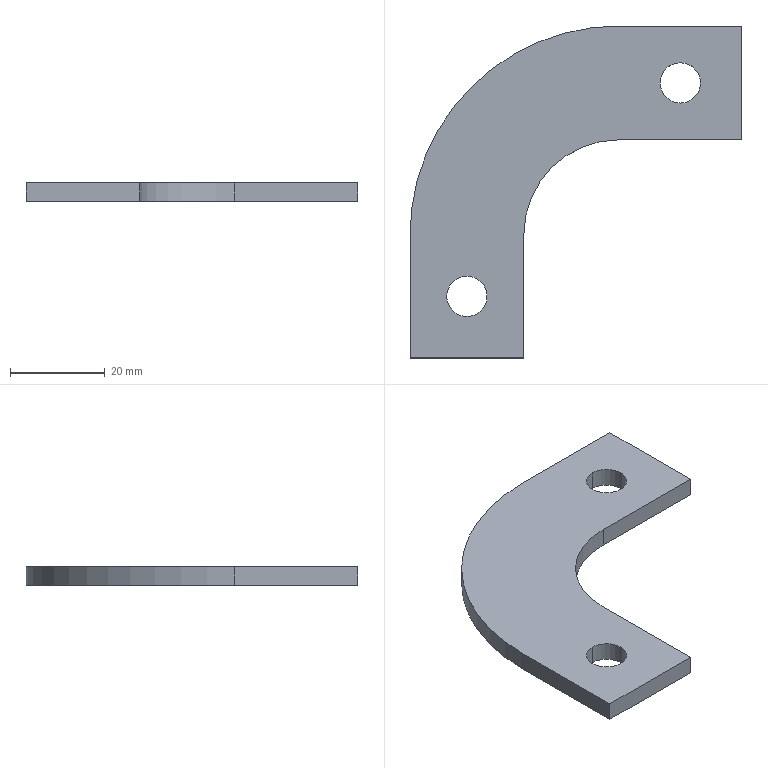Part | SolidWorks | features BaseBody 1 | 1 solid | 14 faces | box 70 x 70 x 4 mm | volume 9364 mm3 | plane 8 | cylinder 6 | commonest cylinder face diameters 8.5 x4 40 x1 88 x1
STEP:
#1=CARTESIAN_POINT('',(228.,-30.75,281.));
#2=VERTEX_POINT('',#1);
#3=CARTESIAN_POINT('',(228.,-39.25,281.));
#4=VERTEX_POINT('',#3);
#5=CARTESIAN_POINT('',(228.,-35.,281.));
#6=DIRECTION('',(0.,0.,1.));
#7=DIRECTION('',(0.,1.,0.));
#8=AXIS2_PLACEMENT_3D('',#5,#6,#7);
#9=CIRCLE('',#8,4.25);
#10=EDGE_CURVE('',#2,#4,#9,.T.);
#11=ORIENTED_EDGE('',*,*,#10,.T.);
#12=CARTESIAN_POINT('',(228.,-39.25,277.));
#13=VERTEX_POINT('',#12);
#14=CARTESIAN_POINT('',(228.,-39.25,281.));
#15=DIRECTION('',(0.,0.,-1.));
#16=VECTOR('',#15,1000.);
#17=LINE('',#14,#16);
#18=EDGE_CURVE('',#4,#13,#17,.T.);
#19=ORIENTED_EDGE('',*,*,#18,.T.);
#20=CARTESIAN_POINT('',(228.,-30.75,277.));
#21=VERTEX_POINT('',#20);
#22=CARTESIAN_POINT('',(228.,-35.,277.));
#23=DIRECTION('',(0.,0.,-1.));
#24=DIRECTION('',(0.,-1.,0.));
#25=AXIS2_PLACEMENT_3D('',#22,#23,#24);
#26=CIRCLE('',#25,4.25);
#27=EDGE_CURVE('',#13,#21,#26,.T.);
#28=ORIENTED_EDGE('',*,*,#27,.T.);
#29=CARTESIAN_POINT('',(228.,-30.75,281.));
#30=DIRECTION('',(0.,0.,-1.));
#31=VECTOR('',#30,1000.);
#32=LINE('',#29,#31);
#33=EDGE_CURVE('',#2,#21,#32,.T.);
#34=ORIENTED_EDGE('',*,*,#33,.F.);
#35=EDGE_LOOP('',(#11,#19,#28,#34));
#36=FACE_OUTER_BOUND('',#35,.T.);
#37=CARTESIAN_POINT('',(228.,-35.,281.));
#38=DIRECTION('',(0.,0.,-1.));
#39=DIRECTION('',(0.,1.,0.));
#40=AXIS2_PLACEMENT_3D('',#37,#38,#39);
#41=CYLINDRICAL_SURFACE('',#40,4.25);
#42=ADVANCED_FACE('',(#36),#41,.F.);
#43=CARTESIAN_POINT('',(273.,14.25,281.));
#44=VERTEX_POINT('',#43);
#45=CARTESIAN_POINT('',(273.,5.75,281.));
#46=VERTEX_POINT('',#45);
#47=CARTESIAN_POINT('',(273.,10.,281.));
#48=DIRECTION('',(0.,0.,1.));
#49=DIRECTION('',(0.,1.,0.));
#50=AXIS2_PLACEMENT_3D('',#47,#48,#49);
#51=CIRCLE('',#50,4.25);
#52=EDGE_CURVE('',#44,#46,#51,.T.);
#53=ORIENTED_EDGE('',*,*,#52,.T.);
#54=CARTESIAN_POINT('',(273.,5.75,277.));
#55=VERTEX_POINT('',#54);
#56=CARTESIAN_POINT('',(273.,5.75,281.));
#57=DIRECTION('',(0.,0.,-1.));
#58=VECTOR('',#57,1000.);
#59=LINE('',#56,#58);
#60=EDGE_CURVE('',#46,#55,#59,.T.);
#61=ORIENTED_EDGE('',*,*,#60,.T.);
#62=CARTESIAN_POINT('',(273.,14.25,277.));
#63=VERTEX_POINT('',#62);
#64=CARTESIAN_POINT('',(273.,10.,277.));
#65=DIRECTION('',(0.,0.,-1.));
#66=DIRECTION('',(0.,-1.,0.));
#67=AXIS2_PLACEMENT_3D('',#64,#65,#66);
#68=CIRCLE('',#67,4.25);
#69=EDGE_CURVE('',#55,#63,#68,.T.);
#70=ORIENTED_EDGE('',*,*,#69,.T.);
#71=CARTESIAN_POINT('',(273.,14.25,281.));
#72=DIRECTION('',(0.,0.,-1.));
#73=VECTOR('',#72,1000.);
#74=LINE('',#71,#73);
#75=EDGE_CURVE('',#44,#63,#74,.T.);
#76=ORIENTED_EDGE('',*,*,#75,.F.);
#77=EDGE_LOOP('',(#53,#61,#70,#76));
#78=FACE_OUTER_BOUND('',#77,.T.);
#79=CARTESIAN_POINT('',(273.,10.,281.));
#80=DIRECTION('',(0.,0.,-1.));
#81=DIRECTION('',(0.,1.,0.));
#82=AXIS2_PLACEMENT_3D('',#79,#80,#81);
#83=CYLINDRICAL_SURFACE('',#82,4.25);
#84=ADVANCED_FACE('',(#78),#83,.F.);
#85=CARTESIAN_POINT('',(273.,10.,277.));
#86=DIRECTION('',(0.,0.,-1.));
#87=DIRECTION('',(0.,-1.,0.));
#88=AXIS2_PLACEMENT_3D('',#85,#86,#87);
#89=CIRCLE('',#88,4.25);
#90=EDGE_CURVE('',#63,#55,#89,.T.);
#91=ORIENTED_EDGE('',*,*,#90,.F.);
#92=ORIENTED_EDGE('',*,*,#69,.F.);
#93=EDGE_LOOP('',(#91,#92));
#94=FACE_BOUND('',#93,.T.);
#95=CARTESIAN_POINT('',(228.,-35.,277.));
#96=DIRECTION('',(0.,0.,-1.));
#97=DIRECTION('',(0.,-1.,0.));
#98=AXIS2_PLACEMENT_3D('',#95,#96,#97);
#99=CIRCLE('',#98,4.25);
#100=EDGE_CURVE('',#21,#13,#99,.T.);
#101=ORIENTED_EDGE('',*,*,#100,.F.);
#102=ORIENTED_EDGE('',*,*,#27,.F.);
#103=EDGE_LOOP('',(#101,#102));
#104=FACE_BOUND('',#103,.T.);
#105=CARTESIAN_POINT('',(216.,-48.,277.));
#106=VERTEX_POINT('',#105);
#107=CARTESIAN_POINT('',(240.,-48.,277.));
#108=VERTEX_POINT('',#107);
#109=CARTESIAN_POINT('',(216.,-48.,277.));
#110=DIRECTION('',(1.,0.,0.));
#111=VECTOR('',#110,1000.);
#112=LINE('',#109,#111);
#113=EDGE_CURVE('',#106,#108,#112,.T.);
#114=ORIENTED_EDGE('',*,*,#113,.F.);
#115=CARTESIAN_POINT('',(216.,-22.,277.));
#116=VERTEX_POINT('',#115);
#117=CARTESIAN_POINT('',(216.,-22.,277.));
#118=DIRECTION('',(0.,-1.,0.));
#119=VECTOR('',#118,1000.);
#120=LINE('',#117,#119);
#121=EDGE_CURVE('',#116,#106,#120,.T.);
#122=ORIENTED_EDGE('',*,*,#121,.F.);
#123=CARTESIAN_POINT('',(260.,22.,277.));
#124=VERTEX_POINT('',#123);
#125=CARTESIAN_POINT('',(260.,-22.,277.));
#126=DIRECTION('',(0.,0.,1.));
#127=DIRECTION('',(0.,1.,0.));
#128=AXIS2_PLACEMENT_3D('',#125,#126,#127);
#129=CIRCLE('',#128,44.);
#130=EDGE_CURVE('',#124,#116,#129,.T.);
#131=ORIENTED_EDGE('',*,*,#130,.F.);
#132=CARTESIAN_POINT('',(286.,22.,277.));
#133=VERTEX_POINT('',#132);
#134=CARTESIAN_POINT('',(286.,22.,277.));
#135=DIRECTION('',(-1.,0.,0.));
#136=VECTOR('',#135,1000.);
#137=LINE('',#134,#136);
#138=EDGE_CURVE('',#133,#124,#137,.T.);
#139=ORIENTED_EDGE('',*,*,#138,.F.);
#140=CARTESIAN_POINT('',(286.,-2.,277.));
#141=VERTEX_POINT('',#140);
#142=CARTESIAN_POINT('',(286.,-2.,277.));
#143=DIRECTION('',(0.,1.,0.));
#144=VECTOR('',#143,1000.);
#145=LINE('',#142,#144);
#146=EDGE_CURVE('',#141,#133,#145,.T.);
#147=ORIENTED_EDGE('',*,*,#146,.F.);
#148=CARTESIAN_POINT('',(260.,-2.,277.));
#149=VERTEX_POINT('',#148);
#150=CARTESIAN_POINT('',(260.,-2.,277.));
#151=DIRECTION('',(1.,0.,0.));
#152=VECTOR('',#151,1000.);
#153=LINE('',#150,#152);
#154=EDGE_CURVE('',#149,#141,#153,.T.);
#155=ORIENTED_EDGE('',*,*,#154,.F.);
#156=CARTESIAN_POINT('',(240.,-22.,277.));
#157=VERTEX_POINT('',#156);
#158=CARTESIAN_POINT('',(260.,-22.,277.));
#159=DIRECTION('',(0.,0.,-1.));
#160=DIRECTION('',(-1.,0.,0.));
#161=AXIS2_PLACEMENT_3D('',#158,#159,#160);
#162=CIRCLE('',#161,20.);
#163=EDGE_CURVE('',#157,#149,#162,.T.);
#164=ORIENTED_EDGE('',*,*,#163,.F.);
#165=CARTESIAN_POINT('',(240.,-48.,277.));
#166=DIRECTION('',(0.,1.,0.));
#167=VECTOR('',#166,1000.);
#168=LINE('',#165,#167);
#169=EDGE_CURVE('',#108,#157,#168,.T.);
#170=ORIENTED_EDGE('',*,*,#169,.F.);
#171=EDGE_LOOP('',(#114,#122,#131,#139,#147,#155,#164,#170));
#172=FACE_OUTER_BOUND('',#171,.T.);
#173=CARTESIAN_POINT('',(260.,-22.,277.));
#174=DIRECTION('',(0.,0.,-1.));
#175=DIRECTION('',(-1.,0.,0.));
#176=AXIS2_PLACEMENT_3D('',#173,#174,#175);
#177=PLANE('',#176);
#178=ADVANCED_FACE('',(#94,#104,#172),#177,.T.);
#179=ORIENTED_EDGE('',*,*,#52,.F.);
#180=CARTESIAN_POINT('',(273.,10.,281.));
#181=DIRECTION('',(0.,0.,1.));
#182=DIRECTION('',(0.,1.,0.));
#183=AXIS2_PLACEMENT_3D('',#180,#181,#182);
#184=CIRCLE('',#183,4.25);
#185=EDGE_CURVE('',#46,#44,#184,.T.);
#186=ORIENTED_EDGE('',*,*,#185,.F.);
#187=EDGE_LOOP('',(#179,#186));
#188=FACE_BOUND('',#187,.T.);
#189=ORIENTED_EDGE('',*,*,#10,.F.);
#190=CARTESIAN_POINT('',(228.,-35.,281.));
#191=DIRECTION('',(0.,0.,1.));
#192=DIRECTION('',(0.,1.,0.));
#193=AXIS2_PLACEMENT_3D('',#190,#191,#192);
#194=CIRCLE('',#193,4.25);
#195=EDGE_CURVE('',#4,#2,#194,.T.);
#196=ORIENTED_EDGE('',*,*,#195,.F.);
#197=EDGE_LOOP('',(#189,#196));
#198=FACE_BOUND('',#197,.T.);
#199=CARTESIAN_POINT('',(240.,-48.,281.));
#200=VERTEX_POINT('',#199);
#201=CARTESIAN_POINT('',(216.,-48.,281.));
#202=VERTEX_POINT('',#201);
#203=CARTESIAN_POINT('',(240.,-48.,281.));
#204=DIRECTION('',(-1.,0.,0.));
#205=VECTOR('',#204,1000.);
#206=LINE('',#203,#205);
#207=EDGE_CURVE('',#200,#202,#206,.T.);
#208=ORIENTED_EDGE('',*,*,#207,.F.);
#209=CARTESIAN_POINT('',(240.,-22.,281.));
#210=VERTEX_POINT('',#209);
#211=CARTESIAN_POINT('',(240.,-22.,281.));
#212=DIRECTION('',(0.,-1.,0.));
#213=VECTOR('',#212,1000.);
#214=LINE('',#211,#213);
#215=EDGE_CURVE('',#210,#200,#214,.T.);
#216=ORIENTED_EDGE('',*,*,#215,.F.);
#217=CARTESIAN_POINT('',(260.,-2.,281.));
#218=VERTEX_POINT('',#217);
#219=CARTESIAN_POINT('',(260.,-22.,281.));
#220=DIRECTION('',(0.,0.,1.));
#221=DIRECTION('',(0.,1.,0.));
#222=AXIS2_PLACEMENT_3D('',#219,#220,#221);
#223=CIRCLE('',#222,20.);
#224=EDGE_CURVE('',#218,#210,#223,.T.);
#225=ORIENTED_EDGE('',*,*,#224,.F.);
#226=CARTESIAN_POINT('',(286.,-2.,281.));
#227=VERTEX_POINT('',#226);
#228=CARTESIAN_POINT('',(286.,-2.,281.));
#229=DIRECTION('',(-1.,0.,0.));
#230=VECTOR('',#229,1000.);
#231=LINE('',#228,#230);
#232=EDGE_CURVE('',#227,#218,#231,.T.);
#233=ORIENTED_EDGE('',*,*,#232,.F.);
#234=CARTESIAN_POINT('',(286.,22.,281.));
#235=VERTEX_POINT('',#234);
#236=CARTESIAN_POINT('',(286.,22.,281.));
#237=DIRECTION('',(0.,-1.,0.));
#238=VECTOR('',#237,1000.);
#239=LINE('',#236,#238);
#240=EDGE_CURVE('',#235,#227,#239,.T.);
#241=ORIENTED_EDGE('',*,*,#240,.F.);
#242=CARTESIAN_POINT('',(260.,22.,281.));
#243=VERTEX_POINT('',#242);
#244=CARTESIAN_POINT('',(260.,22.,281.));
#245=DIRECTION('',(1.,0.,0.));
#246=VECTOR('',#245,1000.);
#247=LINE('',#244,#246);
#248=EDGE_CURVE('',#243,#235,#247,.T.);
#249=ORIENTED_EDGE('',*,*,#248,.F.);
#250=CARTESIAN_POINT('',(216.,-22.,281.));
#251=VERTEX_POINT('',#250);
#252=CARTESIAN_POINT('',(260.,-22.,281.));
#253=DIRECTION('',(0.,0.,-1.));
#254=DIRECTION('',(-1.,0.,0.));
#255=AXIS2_PLACEMENT_3D('',#252,#253,#254);
#256=CIRCLE('',#255,44.);
#257=EDGE_CURVE('',#251,#243,#256,.T.);
#258=ORIENTED_EDGE('',*,*,#257,.F.);
#259=CARTESIAN_POINT('',(216.,-48.,281.));
#260=DIRECTION('',(0.,1.,0.));
#261=VECTOR('',#260,1000.);
#262=LINE('',#259,#261);
#263=EDGE_CURVE('',#202,#251,#262,.T.);
#264=ORIENTED_EDGE('',*,*,#263,.F.);
#265=EDGE_LOOP('',(#208,#216,#225,#233,#241,#249,#258,#264));
#266=FACE_OUTER_BOUND('',#265,.T.);
#267=CARTESIAN_POINT('',(260.,-22.,281.));
#268=DIRECTION('',(0.,0.,1.));
#269=DIRECTION('',(0.,-1.,0.));
#270=AXIS2_PLACEMENT_3D('',#267,#268,#269);
#271=PLANE('',#270);
#272=ADVANCED_FACE('',(#188,#198,#266),#271,.T.);
#273=ORIENTED_EDGE('',*,*,#60,.F.);
#274=ORIENTED_EDGE('',*,*,#185,.T.);
#275=ORIENTED_EDGE('',*,*,#75,.T.);
#276=ORIENTED_EDGE('',*,*,#90,.T.);
#277=EDGE_LOOP('',(#273,#274,#275,#276));
#278=FACE_OUTER_BOUND('',#277,.T.);
#279=CARTESIAN_POINT('',(273.,10.,281.));
#280=DIRECTION('',(0.,0.,-1.));
#281=DIRECTION('',(0.,1.,0.));
#282=AXIS2_PLACEMENT_3D('',#279,#280,#281);
#283=CYLINDRICAL_SURFACE('',#282,4.25);
#284=ADVANCED_FACE('',(#278),#283,.F.);
#285=ORIENTED_EDGE('',*,*,#121,.T.);
#286=CARTESIAN_POINT('',(216.,-48.,281.));
#287=DIRECTION('',(0.,0.,-1.));
#288=VECTOR('',#287,1000.);
#289=LINE('',#286,#288);
#290=EDGE_CURVE('',#202,#106,#289,.T.);
#291=ORIENTED_EDGE('',*,*,#290,.F.);
#292=ORIENTED_EDGE('',*,*,#263,.T.);
#293=CARTESIAN_POINT('',(216.,-22.,277.));
#294=DIRECTION('',(0.,0.,1.));
#295=VECTOR('',#294,1000.);
#296=LINE('',#293,#295);
#297=EDGE_CURVE('',#116,#251,#296,.T.);
#298=ORIENTED_EDGE('',*,*,#297,.F.);
#299=EDGE_LOOP('',(#285,#291,#292,#298));
#300=FACE_OUTER_BOUND('',#299,.T.);
#301=CARTESIAN_POINT('',(216.,-22.,281.));
#302=DIRECTION('',(-1.,0.,0.));
#303=DIRECTION('',(0.,0.,1.));
#304=AXIS2_PLACEMENT_3D('',#301,#302,#303);
#305=PLANE('',#304);
#306=ADVANCED_FACE('',(#300),#305,.T.);
#307=ORIENTED_EDGE('',*,*,#18,.F.);
#308=ORIENTED_EDGE('',*,*,#195,.T.);
#309=ORIENTED_EDGE('',*,*,#33,.T.);
#310=ORIENTED_EDGE('',*,*,#100,.T.);
#311=EDGE_LOOP('',(#307,#308,#309,#310));
#312=FACE_OUTER_BOUND('',#311,.T.);
#313=CARTESIAN_POINT('',(228.,-35.,281.));
#314=DIRECTION('',(0.,0.,-1.));
#315=DIRECTION('',(0.,1.,0.));
#316=AXIS2_PLACEMENT_3D('',#313,#314,#315);
#317=CYLINDRICAL_SURFACE('',#316,4.25);
#318=ADVANCED_FACE('',(#312),#317,.F.);
#319=ORIENTED_EDGE('',*,*,#130,.T.);
#320=ORIENTED_EDGE('',*,*,#297,.T.);
#321=ORIENTED_EDGE('',*,*,#257,.T.);
#322=CARTESIAN_POINT('',(260.,22.,277.));
#323=DIRECTION('',(0.,0.,1.));
#324=VECTOR('',#323,1000.);
#325=LINE('',#322,#324);
#326=EDGE_CURVE('',#124,#243,#325,.T.);
#327=ORIENTED_EDGE('',*,*,#326,.F.);
#328=EDGE_LOOP('',(#319,#320,#321,#327));
#329=FACE_OUTER_BOUND('',#328,.T.);
#330=CARTESIAN_POINT('',(260.,-22.,281.));
#331=DIRECTION('',(0.,0.,-1.));
#332=DIRECTION('',(0.,-1.,0.));
#333=AXIS2_PLACEMENT_3D('',#330,#331,#332);
#334=CYLINDRICAL_SURFACE('',#333,44.);
#335=ADVANCED_FACE('',(#329),#334,.T.);
#336=ORIENTED_EDGE('',*,*,#138,.T.);
#337=ORIENTED_EDGE('',*,*,#326,.T.);
#338=ORIENTED_EDGE('',*,*,#248,.T.);
#339=CARTESIAN_POINT('',(286.,22.,277.));
#340=DIRECTION('',(0.,0.,1.));
#341=VECTOR('',#340,1000.);
#342=LINE('',#339,#341);
#343=EDGE_CURVE('',#133,#235,#342,.T.);
#344=ORIENTED_EDGE('',*,*,#343,.F.);
#345=EDGE_LOOP('',(#336,#337,#338,#344));
#346=FACE_OUTER_BOUND('',#345,.T.);
#347=CARTESIAN_POINT('',(286.,22.,281.));
#348=DIRECTION('',(0.,1.,0.));
#349=DIRECTION('',(0.,0.,-1.));
#350=AXIS2_PLACEMENT_3D('',#347,#348,#349);
#351=PLANE('',#350);
#352=ADVANCED_FACE('',(#346),#351,.T.);
#353=ORIENTED_EDGE('',*,*,#146,.T.);
#354=ORIENTED_EDGE('',*,*,#343,.T.);
#355=ORIENTED_EDGE('',*,*,#240,.T.);
#356=CARTESIAN_POINT('',(286.,-2.,277.));
#357=DIRECTION('',(0.,0.,1.));
#358=VECTOR('',#357,1000.);
#359=LINE('',#356,#358);
#360=EDGE_CURVE('',#141,#227,#359,.T.);
#361=ORIENTED_EDGE('',*,*,#360,.F.);
#362=EDGE_LOOP('',(#353,#354,#355,#361));
#363=FACE_OUTER_BOUND('',#362,.T.);
#364=CARTESIAN_POINT('',(286.,-2.,281.));
#365=DIRECTION('',(1.,0.,0.));
#366=DIRECTION('',(0.,-1.,0.));
#367=AXIS2_PLACEMENT_3D('',#364,#365,#366);
#368=PLANE('',#367);
#369=ADVANCED_FACE('',(#363),#368,.T.);
#370=ORIENTED_EDGE('',*,*,#154,.T.);
#371=ORIENTED_EDGE('',*,*,#360,.T.);
#372=ORIENTED_EDGE('',*,*,#232,.T.);
#373=CARTESIAN_POINT('',(260.,-2.,277.));
#374=DIRECTION('',(0.,0.,1.));
#375=VECTOR('',#374,1000.);
#376=LINE('',#373,#375);
#377=EDGE_CURVE('',#149,#218,#376,.T.);
#378=ORIENTED_EDGE('',*,*,#377,.F.);
#379=EDGE_LOOP('',(#370,#371,#372,#378));
#380=FACE_OUTER_BOUND('',#379,.T.);
#381=CARTESIAN_POINT('',(260.,-2.,281.));
#382=DIRECTION('',(0.,-1.,0.));
#383=DIRECTION('',(0.,0.,-1.));
#384=AXIS2_PLACEMENT_3D('',#381,#382,#383);
#385=PLANE('',#384);
#386=ADVANCED_FACE('',(#380),#385,.T.);
#387=ORIENTED_EDGE('',*,*,#163,.T.);
#388=ORIENTED_EDGE('',*,*,#377,.T.);
#389=ORIENTED_EDGE('',*,*,#224,.T.);
#390=CARTESIAN_POINT('',(240.,-22.,277.));
#391=DIRECTION('',(0.,0.,1.));
#392=VECTOR('',#391,1000.);
#393=LINE('',#390,#392);
#394=EDGE_CURVE('',#157,#210,#393,.T.);
#395=ORIENTED_EDGE('',*,*,#394,.F.);
#396=EDGE_LOOP('',(#387,#388,#389,#395));
#397=FACE_OUTER_BOUND('',#396,.T.);
#398=CARTESIAN_POINT('',(260.,-22.,281.));
#399=DIRECTION('',(0.,0.,-1.));
#400=DIRECTION('',(1.,0.,0.));
#401=AXIS2_PLACEMENT_3D('',#398,#399,#400);
#402=CYLINDRICAL_SURFACE('',#401,20.);
#403=ADVANCED_FACE('',(#397),#402,.F.);
#404=ORIENTED_EDGE('',*,*,#169,.T.);
#405=ORIENTED_EDGE('',*,*,#394,.T.);
#406=ORIENTED_EDGE('',*,*,#215,.T.);
#407=CARTESIAN_POINT('',(240.,-48.,277.));
#408=DIRECTION('',(0.,0.,1.));
#409=VECTOR('',#408,1000.);
#410=LINE('',#407,#409);
#411=EDGE_CURVE('',#108,#200,#410,.T.);
#412=ORIENTED_EDGE('',*,*,#411,.F.);
#413=EDGE_LOOP('',(#404,#405,#406,#412));
#414=FACE_OUTER_BOUND('',#413,.T.);
#415=CARTESIAN_POINT('',(240.,-48.,281.));
#416=DIRECTION('',(1.,0.,0.));
#417=DIRECTION('',(0.,-1.,0.));
#418=AXIS2_PLACEMENT_3D('',#415,#416,#417);
#419=PLANE('',#418);
#420=ADVANCED_FACE('',(#414),#419,.T.);
#421=ORIENTED_EDGE('',*,*,#113,.T.);
#422=ORIENTED_EDGE('',*,*,#411,.T.);
#423=ORIENTED_EDGE('',*,*,#207,.T.);
#424=ORIENTED_EDGE('',*,*,#290,.T.);
#425=EDGE_LOOP('',(#421,#422,#423,#424));
#426=FACE_OUTER_BOUND('',#425,.T.);
#427=CARTESIAN_POINT('',(216.,-48.,281.));
#428=DIRECTION('',(0.,-1.,0.));
#429=DIRECTION('',(0.,0.,-1.));
#430=AXIS2_PLACEMENT_3D('',#427,#428,#429);
#431=PLANE('',#430);
#432=ADVANCED_FACE('',(#426),#431,.T.);
#433=CLOSED_SHELL('',(#42,#84,#178,#272,#284,#306,#318,#335,#352,#369,#386,#403,#420,#432));
#434=MANIFOLD_SOLID_BREP('',#433);
#435=CARTESIAN_POINT('',(0.,0.,0.));
#436=DIRECTION('',(0.,0.,1.));
#437=DIRECTION('',(1.,0.,0.));
#438=AXIS2_PLACEMENT_3D('',#435,#436,#437);
#439=(LENGTH_UNIT()NAMED_UNIT(*)SI_UNIT(.MILLI.,.METRE.));
#440=UNCERTAINTY_MEASURE_WITH_UNIT(LENGTH_MEASURE(0.00001),#439,'','');
#441=(NAMED_UNIT(*)PLANE_ANGLE_UNIT()SI_UNIT($,.RADIAN.));
#442=(NAMED_UNIT(*)SI_UNIT($,.STERADIAN.)SOLID_ANGLE_UNIT());
#443=(GEOMETRIC_REPRESENTATION_CONTEXT(3)GLOBAL_UNCERTAINTY_ASSIGNED_CONTEXT((#440))GLOBAL_UNIT_ASSIGNED_CONTEXT((#439,#441,#442))REPRESENTATION_CONTEXT('',''));
#444=ADVANCED_BREP_SHAPE_REPRESENTATION('',(#434,#438),#443);